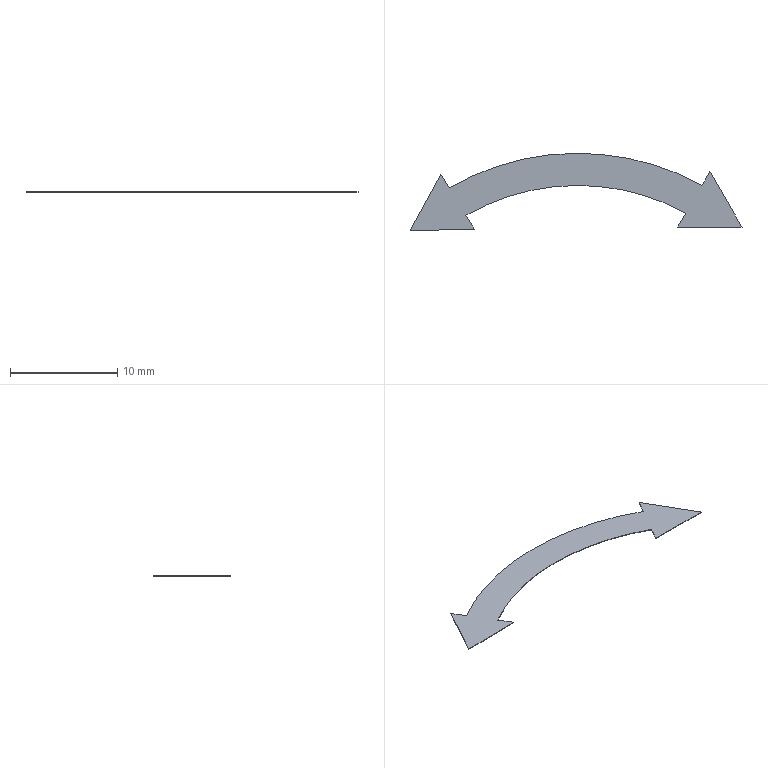Part | STEP file | J101-EBZ05-17-12-Part-1 | 1 solid | 12 faces | box 30.976 x 7.216 x 0.05 mm | volume 5.016 mm3 | plane 10 | cylinder 2 | commonest cylinder face diameters 41.852 x1 47.852 x1
STEP:
#1=CARTESIAN_POINT('',(0.,0.,0.));
#2=DIRECTION('',(0.,0.,1.));
#3=DIRECTION('',(1.,0.,0.));
#4=AXIS2_PLACEMENT_3D('',#1,#2,#3);
#5=CARTESIAN_POINT('',(12.575,12.982,0.));
#6=VERTEX_POINT('',#5);
#7=CARTESIAN_POINT('',(11.822,11.684,0.));
#8=VERTEX_POINT('',#7);
#9=CARTESIAN_POINT('',(12.575,12.982,0.));
#10=DIRECTION('',(-0.5021,-0.8648,0.));
#11=VECTOR('',#10,1.);
#12=LINE('',#9,#11);
#13=CARTESIAN_POINT('',(12.575,12.982,0.05));
#14=DIRECTION('',(0.8648,-0.5021,0.));
#15=DIRECTION('',(0.5021,0.8648,0.));
#16=AXIS2_PLACEMENT_3D('',#13,#14,#15);
#17=PLANE('',#16);
#18=CARTESIAN_POINT('',(0.,-0.05));
#19=DIRECTION('',(-1.,0.));
#20=VECTOR('',#19,1.);
#21=LINE('',#18,#20);
#22=(GEOMETRIC_REPRESENTATION_CONTEXT(2)PARAMETRIC_REPRESENTATION_CONTEXT()REPRESENTATION_CONTEXT('',''));
#23=DEFINITIONAL_REPRESENTATION('',(#21),#22);
#24=PCURVE('',#17,#23);
#25=CARTESIAN_POINT('',(0.2533,-9.259,0.));
#26=DIRECTION('',(0.,0.,1.));
#27=DIRECTION('',(1.,0.,0.));
#28=AXIS2_PLACEMENT_3D('',#25,#26,#27);
#29=PLANE('',#28);
#30=CARTESIAN_POINT('',(12.322,22.241));
#31=DIRECTION('',(-0.5021,-0.8648));
#32=VECTOR('',#31,1.);
#33=LINE('',#30,#32);
#34=(GEOMETRIC_REPRESENTATION_CONTEXT(2)PARAMETRIC_REPRESENTATION_CONTEXT()REPRESENTATION_CONTEXT('',''));
#35=DEFINITIONAL_REPRESENTATION('',(#33),#34);
#36=PCURVE('',#29,#35);
#37=SURFACE_CURVE('',#12,(#24,#36),.PCURVE_S1.);
#38=EDGE_CURVE('',#6,#8,#37,.T.);
#39=ORIENTED_EDGE('',*,*,#38,.T.);
#40=CARTESIAN_POINT('',(11.822,11.684,0.05));
#41=VERTEX_POINT('',#40);
#42=CARTESIAN_POINT('',(11.822,11.684,0.05));
#43=DIRECTION('',(0.,0.,-1.));
#44=VECTOR('',#43,1.);
#45=LINE('',#42,#44);
#46=CARTESIAN_POINT('',(-1.5,0.));
#47=DIRECTION('',(0.,-1.));
#48=VECTOR('',#47,1.);
#49=LINE('',#46,#48);
#50=(GEOMETRIC_REPRESENTATION_CONTEXT(2)PARAMETRIC_REPRESENTATION_CONTEXT()REPRESENTATION_CONTEXT('',''));
#51=DEFINITIONAL_REPRESENTATION('',(#49),#50);
#52=PCURVE('',#17,#51);
#53=CARTESIAN_POINT('',(0.2533,-9.259,0.05));
#54=DIRECTION('',(0.,0.,-1.));
#55=DIRECTION('',(-1.,0.,0.));
#56=AXIS2_PLACEMENT_3D('',#53,#54,#55);
#57=CYLINDRICAL_SURFACE('',#56,23.926);
#58=CARTESIAN_POINT('',(2.075,0.));
#59=DIRECTION('',(0.,1.));
#60=VECTOR('',#59,1.);
#61=LINE('',#58,#60);
#62=(GEOMETRIC_REPRESENTATION_CONTEXT(2)PARAMETRIC_REPRESENTATION_CONTEXT()REPRESENTATION_CONTEXT('',''));
#63=DEFINITIONAL_REPRESENTATION('',(#61),#62);
#64=PCURVE('',#57,#63);
#65=SURFACE_CURVE('',#45,(#52,#64),.PCURVE_S1.);
#66=EDGE_CURVE('',#41,#8,#65,.T.);
#67=ORIENTED_EDGE('',*,*,#66,.F.);
#68=CARTESIAN_POINT('',(12.575,12.982,0.05));
#69=VERTEX_POINT('',#68);
#70=CARTESIAN_POINT('',(12.575,12.982,0.05));
#71=DIRECTION('',(-0.5021,-0.8648,0.));
#72=VECTOR('',#71,1.);
#73=LINE('',#70,#72);
#74=CARTESIAN_POINT('',(0.,0.));
#75=DIRECTION('',(-1.,0.));
#76=VECTOR('',#75,1.);
#77=LINE('',#74,#76);
#78=(GEOMETRIC_REPRESENTATION_CONTEXT(2)PARAMETRIC_REPRESENTATION_CONTEXT()REPRESENTATION_CONTEXT('',''));
#79=DEFINITIONAL_REPRESENTATION('',(#77),#78);
#80=PCURVE('',#17,#79);
#81=CARTESIAN_POINT('',(0.2533,-9.259,0.05));
#82=DIRECTION('',(0.,0.,1.));
#83=DIRECTION('',(1.,0.,0.));
#84=AXIS2_PLACEMENT_3D('',#81,#82,#83);
#85=PLANE('',#84);
#86=CARTESIAN_POINT('',(12.322,22.241));
#87=DIRECTION('',(-0.5021,-0.8648));
#88=VECTOR('',#87,1.);
#89=LINE('',#86,#88);
#90=(GEOMETRIC_REPRESENTATION_CONTEXT(2)PARAMETRIC_REPRESENTATION_CONTEXT()REPRESENTATION_CONTEXT('',''));
#91=DEFINITIONAL_REPRESENTATION('',(#89),#90);
#92=PCURVE('',#85,#91);
#93=SURFACE_CURVE('',#73,(#80,#92),.PCURVE_S1.);
#94=EDGE_CURVE('',#69,#41,#93,.T.);
#95=ORIENTED_EDGE('',*,*,#94,.F.);
#96=CARTESIAN_POINT('',(12.575,12.982,0.05));
#97=DIRECTION('',(0.,0.,-1.));
#98=VECTOR('',#97,1.);
#99=LINE('',#96,#98);
#100=CARTESIAN_POINT('',(0.,0.));
#101=DIRECTION('',(0.,-1.));
#102=VECTOR('',#101,1.);
#103=LINE('',#100,#102);
#104=(GEOMETRIC_REPRESENTATION_CONTEXT(2)PARAMETRIC_REPRESENTATION_CONTEXT()REPRESENTATION_CONTEXT('',''));
#105=DEFINITIONAL_REPRESENTATION('',(#103),#104);
#106=PCURVE('',#17,#105);
#107=CARTESIAN_POINT('',(15.564,7.777,0.05));
#108=DIRECTION('',(-0.8672,-0.4979,0.));
#109=DIRECTION('',(0.4979,-0.8672,0.));
#110=AXIS2_PLACEMENT_3D('',#107,#108,#109);
#111=PLANE('',#110);
#112=CARTESIAN_POINT('',(-6.002,0.));
#113=DIRECTION('',(0.,-1.));
#114=VECTOR('',#113,1.);
#115=LINE('',#112,#114);
#116=(GEOMETRIC_REPRESENTATION_CONTEXT(2)PARAMETRIC_REPRESENTATION_CONTEXT()REPRESENTATION_CONTEXT('',''));
#117=DEFINITIONAL_REPRESENTATION('',(#115),#116);
#118=PCURVE('',#111,#117);
#119=SURFACE_CURVE('',#99,(#106,#118),.PCURVE_S1.);
#120=EDGE_CURVE('',#69,#6,#119,.T.);
#121=ORIENTED_EDGE('',*,*,#120,.T.);
#122=EDGE_LOOP('',(#39,#67,#95,#121));
#123=FACE_BOUND('',#122,.T.);
#124=ADVANCED_FACE('',(#123),#17,.F.);
#125=CARTESIAN_POINT('',(-11.754,11.436,0.));
#126=VERTEX_POINT('',#125);
#127=CARTESIAN_POINT('',(0.2533,-9.259,0.));
#128=DIRECTION('',(0.,0.,1.));
#129=DIRECTION('',(1.,0.,0.));
#130=AXIS2_PLACEMENT_3D('',#127,#128,#129);
#131=CIRCLE('',#130,23.926);
#132=CARTESIAN_POINT('',(3.142,0.05));
#133=DIRECTION('',(-1.,0.));
#134=VECTOR('',#133,1.);
#135=LINE('',#132,#134);
#136=(GEOMETRIC_REPRESENTATION_CONTEXT(2)PARAMETRIC_REPRESENTATION_CONTEXT()REPRESENTATION_CONTEXT('',''));
#137=DEFINITIONAL_REPRESENTATION('',(#135),#136);
#138=PCURVE('',#57,#137);
#139=CARTESIAN_POINT('',(0.,0.));
#140=DIRECTION('',(1.,0.));
#141=AXIS2_PLACEMENT_2D('',#139,#140);
#142=CIRCLE('',#141,23.926);
#143=(GEOMETRIC_REPRESENTATION_CONTEXT(2)PARAMETRIC_REPRESENTATION_CONTEXT()REPRESENTATION_CONTEXT('',''));
#144=DEFINITIONAL_REPRESENTATION('',(#142),#143);
#145=PCURVE('',#29,#144);
#146=SURFACE_CURVE('',#131,(#138,#145),.PCURVE_S1.);
#147=EDGE_CURVE('',#8,#126,#146,.T.);
#148=ORIENTED_EDGE('',*,*,#147,.T.);
#149=CARTESIAN_POINT('',(-11.754,11.436,0.05));
#150=VERTEX_POINT('',#149);
#151=CARTESIAN_POINT('',(-11.754,11.436,0.05));
#152=DIRECTION('',(0.,0.,-1.));
#153=VECTOR('',#152,1.);
#154=LINE('',#151,#153);
#155=CARTESIAN_POINT('',(1.045,0.));
#156=DIRECTION('',(0.,1.));
#157=VECTOR('',#156,1.);
#158=LINE('',#155,#157);
#159=(GEOMETRIC_REPRESENTATION_CONTEXT(2)PARAMETRIC_REPRESENTATION_CONTEXT()REPRESENTATION_CONTEXT('',''));
#160=DEFINITIONAL_REPRESENTATION('',(#158),#159);
#161=PCURVE('',#57,#160);
#162=CARTESIAN_POINT('',(-11.754,11.436,0.05));
#163=DIRECTION('',(-0.8541,-0.5202,0.));
#164=DIRECTION('',(0.5202,-0.8541,0.));
#165=AXIS2_PLACEMENT_3D('',#162,#163,#164);
#166=PLANE('',#165);
#167=CARTESIAN_POINT('',(0.,0.));
#168=DIRECTION('',(0.,-1.));
#169=VECTOR('',#168,1.);
#170=LINE('',#167,#169);
#171=(GEOMETRIC_REPRESENTATION_CONTEXT(2)PARAMETRIC_REPRESENTATION_CONTEXT()REPRESENTATION_CONTEXT('',''));
#172=DEFINITIONAL_REPRESENTATION('',(#170),#171);
#173=PCURVE('',#166,#172);
#174=SURFACE_CURVE('',#154,(#161,#173),.PCURVE_S1.);
#175=EDGE_CURVE('',#150,#126,#174,.T.);
#176=ORIENTED_EDGE('',*,*,#175,.F.);
#177=CARTESIAN_POINT('',(0.2533,-9.259,0.05));
#178=DIRECTION('',(0.,0.,1.));
#179=DIRECTION('',(1.,0.,0.));
#180=AXIS2_PLACEMENT_3D('',#177,#178,#179);
#181=CIRCLE('',#180,23.926);
#182=CARTESIAN_POINT('',(3.142,0.));
#183=DIRECTION('',(-1.,0.));
#184=VECTOR('',#183,1.);
#185=LINE('',#182,#184);
#186=(GEOMETRIC_REPRESENTATION_CONTEXT(2)PARAMETRIC_REPRESENTATION_CONTEXT()REPRESENTATION_CONTEXT('',''));
#187=DEFINITIONAL_REPRESENTATION('',(#185),#186);
#188=PCURVE('',#57,#187);
#189=CARTESIAN_POINT('',(0.,0.));
#190=DIRECTION('',(1.,0.));
#191=AXIS2_PLACEMENT_2D('',#189,#190);
#192=CIRCLE('',#191,23.926);
#193=(GEOMETRIC_REPRESENTATION_CONTEXT(2)PARAMETRIC_REPRESENTATION_CONTEXT()REPRESENTATION_CONTEXT('',''));
#194=DEFINITIONAL_REPRESENTATION('',(#192),#193);
#195=PCURVE('',#85,#194);
#196=SURFACE_CURVE('',#181,(#188,#195),.PCURVE_S1.);
#197=EDGE_CURVE('',#41,#150,#196,.T.);
#198=ORIENTED_EDGE('',*,*,#197,.F.);
#199=ORIENTED_EDGE('',*,*,#66,.T.);
#200=EDGE_LOOP('',(#148,#176,#198,#199));
#201=FACE_BOUND('',#200,.T.);
#202=ADVANCED_FACE('',(#201),#57,.T.);
#203=CARTESIAN_POINT('',(-12.535,12.717,0.));
#204=VERTEX_POINT('',#203);
#205=CARTESIAN_POINT('',(-11.754,11.436,0.));
#206=DIRECTION('',(-0.5202,0.8541,0.));
#207=VECTOR('',#206,1.);
#208=LINE('',#205,#207);
#209=CARTESIAN_POINT('',(0.,-0.05));
#210=DIRECTION('',(-1.,0.));
#211=VECTOR('',#210,1.);
#212=LINE('',#209,#211);
#213=(GEOMETRIC_REPRESENTATION_CONTEXT(2)PARAMETRIC_REPRESENTATION_CONTEXT()REPRESENTATION_CONTEXT('',''));
#214=DEFINITIONAL_REPRESENTATION('',(#212),#213);
#215=PCURVE('',#166,#214);
#216=CARTESIAN_POINT('',(-12.007,20.695));
#217=DIRECTION('',(-0.5202,0.8541));
#218=VECTOR('',#217,1.);
#219=LINE('',#216,#218);
#220=(GEOMETRIC_REPRESENTATION_CONTEXT(2)PARAMETRIC_REPRESENTATION_CONTEXT()REPRESENTATION_CONTEXT('',''));
#221=DEFINITIONAL_REPRESENTATION('',(#219),#220);
#222=PCURVE('',#29,#221);
#223=SURFACE_CURVE('',#208,(#215,#222),.PCURVE_S1.);
#224=EDGE_CURVE('',#126,#204,#223,.T.);
#225=ORIENTED_EDGE('',*,*,#224,.T.);
#226=CARTESIAN_POINT('',(-12.535,12.717,0.05));
#227=VERTEX_POINT('',#226);
#228=CARTESIAN_POINT('',(-12.535,12.717,0.05));
#229=DIRECTION('',(0.,0.,-1.));
#230=VECTOR('',#229,1.);
#231=LINE('',#228,#230);
#232=CARTESIAN_POINT('',(-1.5,0.));
#233=DIRECTION('',(0.,-1.));
#234=VECTOR('',#233,1.);
#235=LINE('',#232,#234);
#236=(GEOMETRIC_REPRESENTATION_CONTEXT(2)PARAMETRIC_REPRESENTATION_CONTEXT()REPRESENTATION_CONTEXT('',''));
#237=DEFINITIONAL_REPRESENTATION('',(#235),#236);
#238=PCURVE('',#166,#237);
#239=CARTESIAN_POINT('',(-12.535,12.717,0.05));
#240=DIRECTION('',(0.8775,-0.4795,0.));
#241=DIRECTION('',(0.4795,0.8775,0.));
#242=AXIS2_PLACEMENT_3D('',#239,#240,#241);
#243=PLANE('',#242);
#244=CARTESIAN_POINT('',(0.,0.));
#245=DIRECTION('',(0.,-1.));
#246=VECTOR('',#245,1.);
#247=LINE('',#244,#246);
#248=(GEOMETRIC_REPRESENTATION_CONTEXT(2)PARAMETRIC_REPRESENTATION_CONTEXT()REPRESENTATION_CONTEXT('',''));
#249=DEFINITIONAL_REPRESENTATION('',(#247),#248);
#250=PCURVE('',#243,#249);
#251=SURFACE_CURVE('',#231,(#238,#250),.PCURVE_S1.);
#252=EDGE_CURVE('',#227,#204,#251,.T.);
#253=ORIENTED_EDGE('',*,*,#252,.F.);
#254=CARTESIAN_POINT('',(-11.754,11.436,0.05));
#255=DIRECTION('',(-0.5202,0.8541,0.));
#256=VECTOR('',#255,1.);
#257=LINE('',#254,#256);
#258=CARTESIAN_POINT('',(0.,0.));
#259=DIRECTION('',(-1.,0.));
#260=VECTOR('',#259,1.);
#261=LINE('',#258,#260);
#262=(GEOMETRIC_REPRESENTATION_CONTEXT(2)PARAMETRIC_REPRESENTATION_CONTEXT()REPRESENTATION_CONTEXT('',''));
#263=DEFINITIONAL_REPRESENTATION('',(#261),#262);
#264=PCURVE('',#166,#263);
#265=CARTESIAN_POINT('',(-12.007,20.695));
#266=DIRECTION('',(-0.5202,0.8541));
#267=VECTOR('',#266,1.);
#268=LINE('',#265,#267);
#269=(GEOMETRIC_REPRESENTATION_CONTEXT(2)PARAMETRIC_REPRESENTATION_CONTEXT()REPRESENTATION_CONTEXT('',''));
#270=DEFINITIONAL_REPRESENTATION('',(#268),#269);
#271=PCURVE('',#85,#270);
#272=SURFACE_CURVE('',#257,(#264,#271),.PCURVE_S1.);
#273=EDGE_CURVE('',#150,#227,#272,.T.);
#274=ORIENTED_EDGE('',*,*,#273,.F.);
#275=ORIENTED_EDGE('',*,*,#175,.T.);
#276=EDGE_LOOP('',(#225,#253,#274,#275));
#277=FACE_BOUND('',#276,.T.);
#278=ADVANCED_FACE('',(#277),#166,.F.);
#279=CARTESIAN_POINT('',(-15.413,7.451,0.));
#280=VERTEX_POINT('',#279);
#281=CARTESIAN_POINT('',(-12.535,12.717,0.));
#282=DIRECTION('',(-0.4795,-0.8775,0.));
#283=VECTOR('',#282,1.);
#284=LINE('',#281,#283);
#285=CARTESIAN_POINT('',(0.,-0.05));
#286=DIRECTION('',(-1.,0.));
#287=VECTOR('',#286,1.);
#288=LINE('',#285,#287);
#289=(GEOMETRIC_REPRESENTATION_CONTEXT(2)PARAMETRIC_REPRESENTATION_CONTEXT()REPRESENTATION_CONTEXT('',''));
#290=DEFINITIONAL_REPRESENTATION('',(#288),#289);
#291=PCURVE('',#243,#290);
#292=CARTESIAN_POINT('',(-12.788,21.976));
#293=DIRECTION('',(-0.4795,-0.8775));
#294=VECTOR('',#293,1.);
#295=LINE('',#292,#294);
#296=(GEOMETRIC_REPRESENTATION_CONTEXT(2)PARAMETRIC_REPRESENTATION_CONTEXT()REPRESENTATION_CONTEXT('',''));
#297=DEFINITIONAL_REPRESENTATION('',(#295),#296);
#298=PCURVE('',#29,#297);
#299=SURFACE_CURVE('',#284,(#291,#298),.PCURVE_S1.);
#300=EDGE_CURVE('',#204,#280,#299,.T.);
#301=ORIENTED_EDGE('',*,*,#300,.T.);
#302=CARTESIAN_POINT('',(-15.413,7.451,0.05));
#303=VERTEX_POINT('',#302);
#304=CARTESIAN_POINT('',(-15.413,7.451,0.05));
#305=DIRECTION('',(0.,0.,-1.));
#306=VECTOR('',#305,1.);
#307=LINE('',#304,#306);
#308=CARTESIAN_POINT('',(-6.002,0.));
#309=DIRECTION('',(0.,-1.));
#310=VECTOR('',#309,1.);
#311=LINE('',#308,#310);
#312=(GEOMETRIC_REPRESENTATION_CONTEXT(2)PARAMETRIC_REPRESENTATION_CONTEXT()REPRESENTATION_CONTEXT('',''));
#313=DEFINITIONAL_REPRESENTATION('',(#311),#312);
#314=PCURVE('',#243,#313);
#315=CARTESIAN_POINT('',(-15.413,7.451,0.05));
#316=DIRECTION('',(-0.02346,0.9997,0.));
#317=DIRECTION('',(-0.9997,-0.02346,0.));
#318=AXIS2_PLACEMENT_3D('',#315,#316,#317);
#319=PLANE('',#318);
#320=CARTESIAN_POINT('',(0.,0.));
#321=DIRECTION('',(0.,-1.));
#322=VECTOR('',#321,1.);
#323=LINE('',#320,#322);
#324=(GEOMETRIC_REPRESENTATION_CONTEXT(2)PARAMETRIC_REPRESENTATION_CONTEXT()REPRESENTATION_CONTEXT('',''));
#325=DEFINITIONAL_REPRESENTATION('',(#323),#324);
#326=PCURVE('',#319,#325);
#327=SURFACE_CURVE('',#307,(#314,#326),.PCURVE_S1.);
#328=EDGE_CURVE('',#303,#280,#327,.T.);
#329=ORIENTED_EDGE('',*,*,#328,.F.);
#330=CARTESIAN_POINT('',(-12.535,12.717,0.05));
#331=DIRECTION('',(-0.4795,-0.8775,0.));
#332=VECTOR('',#331,1.);
#333=LINE('',#330,#332);
#334=CARTESIAN_POINT('',(0.,0.));
#335=DIRECTION('',(-1.,0.));
#336=VECTOR('',#335,1.);
#337=LINE('',#334,#336);
#338=(GEOMETRIC_REPRESENTATION_CONTEXT(2)PARAMETRIC_REPRESENTATION_CONTEXT()REPRESENTATION_CONTEXT('',''));
#339=DEFINITIONAL_REPRESENTATION('',(#337),#338);
#340=PCURVE('',#243,#339);
#341=CARTESIAN_POINT('',(-12.788,21.976));
#342=DIRECTION('',(-0.4795,-0.8775));
#343=VECTOR('',#342,1.);
#344=LINE('',#341,#343);
#345=(GEOMETRIC_REPRESENTATION_CONTEXT(2)PARAMETRIC_REPRESENTATION_CONTEXT()REPRESENTATION_CONTEXT('',''));
#346=DEFINITIONAL_REPRESENTATION('',(#344),#345);
#347=PCURVE('',#85,#346);
#348=SURFACE_CURVE('',#333,(#340,#347),.PCURVE_S1.);
#349=EDGE_CURVE('',#227,#303,#348,.T.);
#350=ORIENTED_EDGE('',*,*,#349,.F.);
#351=ORIENTED_EDGE('',*,*,#252,.T.);
#352=EDGE_LOOP('',(#301,#329,#350,#351));
#353=FACE_BOUND('',#352,.T.);
#354=ADVANCED_FACE('',(#353),#243,.F.);
#355=CARTESIAN_POINT('',(-9.413,7.592,0.));
#356=VERTEX_POINT('',#355);
#357=CARTESIAN_POINT('',(-15.413,7.451,0.));
#358=DIRECTION('',(0.9997,0.02346,0.));
#359=VECTOR('',#358,1.);
#360=LINE('',#357,#359);
#361=CARTESIAN_POINT('',(0.,-0.05));
#362=DIRECTION('',(-1.,0.));
#363=VECTOR('',#362,1.);
#364=LINE('',#361,#363);
#365=(GEOMETRIC_REPRESENTATION_CONTEXT(2)PARAMETRIC_REPRESENTATION_CONTEXT()REPRESENTATION_CONTEXT('',''));
#366=DEFINITIONAL_REPRESENTATION('',(#364),#365);
#367=PCURVE('',#319,#366);
#368=CARTESIAN_POINT('',(-15.666,16.71));
#369=DIRECTION('',(0.9997,0.02346));
#370=VECTOR('',#369,1.);
#371=LINE('',#368,#370);
#372=(GEOMETRIC_REPRESENTATION_CONTEXT(2)PARAMETRIC_REPRESENTATION_CONTEXT()REPRESENTATION_CONTEXT('',''));
#373=DEFINITIONAL_REPRESENTATION('',(#371),#372);
#374=PCURVE('',#29,#373);
#375=SURFACE_CURVE('',#360,(#367,#374),.PCURVE_S1.);
#376=EDGE_CURVE('',#280,#356,#375,.T.);
#377=ORIENTED_EDGE('',*,*,#376,.T.);
#378=CARTESIAN_POINT('',(-9.413,7.592,0.05));
#379=VERTEX_POINT('',#378);
#380=CARTESIAN_POINT('',(-9.413,7.592,0.05));
#381=DIRECTION('',(0.,0.,-1.));
#382=VECTOR('',#381,1.);
#383=LINE('',#380,#382);
#384=CARTESIAN_POINT('',(-6.002,0.));
#385=DIRECTION('',(0.,-1.));
#386=VECTOR('',#385,1.);
#387=LINE('',#384,#386);
#388=(GEOMETRIC_REPRESENTATION_CONTEXT(2)PARAMETRIC_REPRESENTATION_CONTEXT()REPRESENTATION_CONTEXT('',''));
#389=DEFINITIONAL_REPRESENTATION('',(#387),#388);
#390=PCURVE('',#319,#389);
#391=CARTESIAN_POINT('',(-9.413,7.592,0.05));
#392=DIRECTION('',(-0.8541,-0.5202,0.));
#393=DIRECTION('',(0.5202,-0.8541,0.));
#394=AXIS2_PLACEMENT_3D('',#391,#392,#393);
#395=PLANE('',#394);
#396=CARTESIAN_POINT('',(0.,0.));
#397=DIRECTION('',(0.,-1.));
#398=VECTOR('',#397,1.);
#399=LINE('',#396,#398);
#400=(GEOMETRIC_REPRESENTATION_CONTEXT(2)PARAMETRIC_REPRESENTATION_CONTEXT()REPRESENTATION_CONTEXT('',''));
#401=DEFINITIONAL_REPRESENTATION('',(#399),#400);
#402=PCURVE('',#395,#401);
#403=SURFACE_CURVE('',#383,(#390,#402),.PCURVE_S1.);
#404=EDGE_CURVE('',#379,#356,#403,.T.);
#405=ORIENTED_EDGE('',*,*,#404,.F.);
#406=CARTESIAN_POINT('',(-15.413,7.451,0.05));
#407=DIRECTION('',(0.9997,0.02346,0.));
#408=VECTOR('',#407,1.);
#409=LINE('',#406,#408);
#410=CARTESIAN_POINT('',(0.,0.));
#411=DIRECTION('',(-1.,0.));
#412=VECTOR('',#411,1.);
#413=LINE('',#410,#412);
#414=(GEOMETRIC_REPRESENTATION_CONTEXT(2)PARAMETRIC_REPRESENTATION_CONTEXT()REPRESENTATION_CONTEXT('',''));
#415=DEFINITIONAL_REPRESENTATION('',(#413),#414);
#416=PCURVE('',#319,#415);
#417=CARTESIAN_POINT('',(-15.666,16.71));
#418=DIRECTION('',(0.9997,0.02346));
#419=VECTOR('',#418,1.);
#420=LINE('',#417,#419);
#421=(GEOMETRIC_REPRESENTATION_CONTEXT(2)PARAMETRIC_REPRESENTATION_CONTEXT()REPRESENTATION_CONTEXT('',''));
#422=DEFINITIONAL_REPRESENTATION('',(#420),#421);
#423=PCURVE('',#85,#422);
#424=SURFACE_CURVE('',#409,(#416,#423),.PCURVE_S1.);
#425=EDGE_CURVE('',#303,#379,#424,.T.);
#426=ORIENTED_EDGE('',*,*,#425,.F.);
#427=ORIENTED_EDGE('',*,*,#328,.T.);
#428=EDGE_LOOP('',(#377,#405,#426,#427));
#429=FACE_BOUND('',#428,.T.);
#430=ADVANCED_FACE('',(#429),#319,.F.);
#431=CARTESIAN_POINT('',(-10.193,8.873,0.));
#432=VERTEX_POINT('',#431);
#433=CARTESIAN_POINT('',(-9.413,7.592,0.));
#434=DIRECTION('',(-0.5202,0.8541,0.));
#435=VECTOR('',#434,1.);
#436=LINE('',#433,#435);
#437=CARTESIAN_POINT('',(0.,-0.05));
#438=DIRECTION('',(-1.,0.));
#439=VECTOR('',#438,1.);
#440=LINE('',#437,#439);
#441=(GEOMETRIC_REPRESENTATION_CONTEXT(2)PARAMETRIC_REPRESENTATION_CONTEXT()REPRESENTATION_CONTEXT('',''));
#442=DEFINITIONAL_REPRESENTATION('',(#440),#441);
#443=PCURVE('',#395,#442);
#444=CARTESIAN_POINT('',(-9.666,16.851));
#445=DIRECTION('',(-0.5202,0.8541));
#446=VECTOR('',#445,1.);
#447=LINE('',#444,#446);
#448=(GEOMETRIC_REPRESENTATION_CONTEXT(2)PARAMETRIC_REPRESENTATION_CONTEXT()REPRESENTATION_CONTEXT('',''));
#449=DEFINITIONAL_REPRESENTATION('',(#447),#448);
#450=PCURVE('',#29,#449);
#451=SURFACE_CURVE('',#436,(#443,#450),.PCURVE_S1.);
#452=EDGE_CURVE('',#356,#432,#451,.T.);
#453=ORIENTED_EDGE('',*,*,#452,.T.);
#454=CARTESIAN_POINT('',(-10.193,8.873,0.05));
#455=VERTEX_POINT('',#454);
#456=CARTESIAN_POINT('',(-10.193,8.873,0.05));
#457=DIRECTION('',(0.,0.,-1.));
#458=VECTOR('',#457,1.);
#459=LINE('',#456,#458);
#460=CARTESIAN_POINT('',(-1.5,0.));
#461=DIRECTION('',(0.,-1.));
#462=VECTOR('',#461,1.);
#463=LINE('',#460,#462);
#464=(GEOMETRIC_REPRESENTATION_CONTEXT(2)PARAMETRIC_REPRESENTATION_CONTEXT()REPRESENTATION_CONTEXT('',''));
#465=DEFINITIONAL_REPRESENTATION('',(#463),#464);
#466=PCURVE('',#395,#465);
#467=CARTESIAN_POINT('',(0.2533,-9.259,0.05));
#468=DIRECTION('',(0.,0.,-1.));
#469=DIRECTION('',(-1.,0.,0.));
#470=AXIS2_PLACEMENT_3D('',#467,#468,#469);
#471=CYLINDRICAL_SURFACE('',#470,20.926);
#472=CARTESIAN_POINT('',(1.048,0.));
#473=DIRECTION('',(0.,1.));
#474=VECTOR('',#473,1.);
#475=LINE('',#472,#474);
#476=(GEOMETRIC_REPRESENTATION_CONTEXT(2)PARAMETRIC_REPRESENTATION_CONTEXT()REPRESENTATION_CONTEXT('',''));
#477=DEFINITIONAL_REPRESENTATION('',(#475),#476);
#478=PCURVE('',#471,#477);
#479=SURFACE_CURVE('',#459,(#466,#478),.PCURVE_S1.);
#480=EDGE_CURVE('',#455,#432,#479,.T.);
#481=ORIENTED_EDGE('',*,*,#480,.F.);
#482=CARTESIAN_POINT('',(-9.413,7.592,0.05));
#483=DIRECTION('',(-0.5202,0.8541,0.));
#484=VECTOR('',#483,1.);
#485=LINE('',#482,#484);
#486=CARTESIAN_POINT('',(0.,0.));
#487=DIRECTION('',(-1.,0.));
#488=VECTOR('',#487,1.);
#489=LINE('',#486,#488);
#490=(GEOMETRIC_REPRESENTATION_CONTEXT(2)PARAMETRIC_REPRESENTATION_CONTEXT()REPRESENTATION_CONTEXT('',''));
#491=DEFINITIONAL_REPRESENTATION('',(#489),#490);
#492=PCURVE('',#395,#491);
#493=CARTESIAN_POINT('',(-9.666,16.851));
#494=DIRECTION('',(-0.5202,0.8541));
#495=VECTOR('',#494,1.);
#496=LINE('',#493,#495);
#497=(GEOMETRIC_REPRESENTATION_CONTEXT(2)PARAMETRIC_REPRESENTATION_CONTEXT()REPRESENTATION_CONTEXT('',''));
#498=DEFINITIONAL_REPRESENTATION('',(#496),#497);
#499=PCURVE('',#85,#498);
#500=SURFACE_CURVE('',#485,(#492,#499),.PCURVE_S1.);
#501=EDGE_CURVE('',#379,#455,#500,.T.);
#502=ORIENTED_EDGE('',*,*,#501,.F.);
#503=ORIENTED_EDGE('',*,*,#404,.T.);
#504=EDGE_LOOP('',(#453,#481,#502,#503));
#505=FACE_BOUND('',#504,.T.);
#506=ADVANCED_FACE('',(#505),#395,.F.);
#507=ORIENTED_EDGE('',*,*,#480,.F.);
#508=CARTESIAN_POINT('',(10.315,9.089,0.05));
#509=VERTEX_POINT('',#508);
#510=CARTESIAN_POINT('',(0.2533,-9.259,0.05));
#511=DIRECTION('',(0.,0.,-1.));
#512=DIRECTION('',(-1.,0.,0.));
#513=AXIS2_PLACEMENT_3D('',#510,#511,#512);
#514=CIRCLE('',#513,20.926);
#515=CARTESIAN_POINT('',(0.,0.));
#516=DIRECTION('',(1.,0.));
#517=VECTOR('',#516,1.);
#518=LINE('',#515,#517);
#519=(GEOMETRIC_REPRESENTATION_CONTEXT(2)PARAMETRIC_REPRESENTATION_CONTEXT()REPRESENTATION_CONTEXT('',''));
#520=DEFINITIONAL_REPRESENTATION('',(#518),#519);
#521=PCURVE('',#471,#520);
#522=CARTESIAN_POINT('',(-20.926,0.));
#523=CARTESIAN_POINT('',(-20.926,36.245));
#524=CARTESIAN_POINT('',(10.463,18.123));
#525=CARTESIAN_POINT('',(41.852,0.));
#526=CARTESIAN_POINT('',(10.463,-18.123));
#527=CARTESIAN_POINT('',(-20.926,-36.245));
#528=CARTESIAN_POINT('',(-20.926,0.));
#529=(BOUNDED_CURVE()B_SPLINE_CURVE(2,(#522,#523,#524,#525,#526,#527,#528),.UNSPECIFIED.,.T.,.F.)B_SPLINE_CURVE_WITH_KNOTS((1,2,2,2,2,1),(-2.094,0.,2.094,4.189,6.283,8.378),.UNSPECIFIED.)CURVE()GEOMETRIC_REPRESENTATION_ITEM()RATIONAL_B_SPLINE_CURVE((1.,0.5,1.,0.5,1.,0.5,1.))REPRESENTATION_ITEM(''));
#530=(GEOMETRIC_REPRESENTATION_CONTEXT(2)PARAMETRIC_REPRESENTATION_CONTEXT()REPRESENTATION_CONTEXT('',''));
#531=DEFINITIONAL_REPRESENTATION('',(#529),#530);
#532=PCURVE('',#85,#531);
#533=SURFACE_CURVE('',#514,(#521,#532),.PCURVE_S1.);
#534=EDGE_CURVE('',#455,#509,#533,.T.);
#535=ORIENTED_EDGE('',*,*,#534,.T.);
#536=CARTESIAN_POINT('',(10.315,9.089,0.));
#537=VERTEX_POINT('',#536);
#538=CARTESIAN_POINT('',(10.315,9.089,0.05));
#539=DIRECTION('',(0.,0.,-1.));
#540=VECTOR('',#539,1.);
#541=LINE('',#538,#540);
#542=CARTESIAN_POINT('',(2.072,0.));
#543=DIRECTION('',(0.,1.));
#544=VECTOR('',#543,1.);
#545=LINE('',#542,#544);
#546=(GEOMETRIC_REPRESENTATION_CONTEXT(2)PARAMETRIC_REPRESENTATION_CONTEXT()REPRESENTATION_CONTEXT('',''));
#547=DEFINITIONAL_REPRESENTATION('',(#545),#546);
#548=PCURVE('',#471,#547);
#549=CARTESIAN_POINT('',(10.315,9.089,0.05));
#550=DIRECTION('',(0.8648,-0.5021,0.));
#551=DIRECTION('',(0.5021,0.8648,0.));
#552=AXIS2_PLACEMENT_3D('',#549,#550,#551);
#553=PLANE('',#552);
#554=CARTESIAN_POINT('',(0.,0.));
#555=DIRECTION('',(0.,-1.));
#556=VECTOR('',#555,1.);
#557=LINE('',#554,#556);
#558=(GEOMETRIC_REPRESENTATION_CONTEXT(2)PARAMETRIC_REPRESENTATION_CONTEXT()REPRESENTATION_CONTEXT('',''));
#559=DEFINITIONAL_REPRESENTATION('',(#557),#558);
#560=PCURVE('',#553,#559);
#561=SURFACE_CURVE('',#541,(#548,#560),.PCURVE_S1.);
#562=EDGE_CURVE('',#509,#537,#561,.T.);
#563=ORIENTED_EDGE('',*,*,#562,.T.);
#564=CARTESIAN_POINT('',(0.2533,-9.259,0.));
#565=DIRECTION('',(0.,0.,-1.));
#566=DIRECTION('',(-1.,0.,0.));
#567=AXIS2_PLACEMENT_3D('',#564,#565,#566);
#568=CIRCLE('',#567,20.926);
#569=CARTESIAN_POINT('',(0.,0.05));
#570=DIRECTION('',(1.,0.));
#571=VECTOR('',#570,1.);
#572=LINE('',#569,#571);
#573=(GEOMETRIC_REPRESENTATION_CONTEXT(2)PARAMETRIC_REPRESENTATION_CONTEXT()REPRESENTATION_CONTEXT('',''));
#574=DEFINITIONAL_REPRESENTATION('',(#572),#573);
#575=PCURVE('',#471,#574);
#576=CARTESIAN_POINT('',(-20.926,0.));
#577=CARTESIAN_POINT('',(-20.926,36.245));
#578=CARTESIAN_POINT('',(10.463,18.123));
#579=CARTESIAN_POINT('',(41.852,0.));
#580=CARTESIAN_POINT('',(10.463,-18.123));
#581=CARTESIAN_POINT('',(-20.926,-36.245));
#582=CARTESIAN_POINT('',(-20.926,0.));
#583=(BOUNDED_CURVE()B_SPLINE_CURVE(2,(#576,#577,#578,#579,#580,#581,#582),.UNSPECIFIED.,.T.,.F.)B_SPLINE_CURVE_WITH_KNOTS((1,2,2,2,2,1),(-2.094,0.,2.094,4.189,6.283,8.378),.UNSPECIFIED.)CURVE()GEOMETRIC_REPRESENTATION_ITEM()RATIONAL_B_SPLINE_CURVE((1.,0.5,1.,0.5,1.,0.5,1.))REPRESENTATION_ITEM(''));
#584=(GEOMETRIC_REPRESENTATION_CONTEXT(2)PARAMETRIC_REPRESENTATION_CONTEXT()REPRESENTATION_CONTEXT('',''));
#585=DEFINITIONAL_REPRESENTATION('',(#583),#584);
#586=PCURVE('',#29,#585);
#587=SURFACE_CURVE('',#568,(#575,#586),.PCURVE_S1.);
#588=EDGE_CURVE('',#432,#537,#587,.T.);
#589=ORIENTED_EDGE('',*,*,#588,.F.);
#590=EDGE_LOOP('',(#507,#535,#563,#589));
#591=FACE_BOUND('',#590,.F.);
#592=ADVANCED_FACE('',(#591),#471,.F.);
#593=CARTESIAN_POINT('',(9.562,7.792,0.));
#594=VERTEX_POINT('',#593);
#595=CARTESIAN_POINT('',(10.315,9.089,0.));
#596=DIRECTION('',(-0.5021,-0.8648,0.));
#597=VECTOR('',#596,1.);
#598=LINE('',#595,#597);
#599=CARTESIAN_POINT('',(0.,-0.05));
#600=DIRECTION('',(-1.,0.));
#601=VECTOR('',#600,1.);
#602=LINE('',#599,#601);
#603=(GEOMETRIC_REPRESENTATION_CONTEXT(2)PARAMETRIC_REPRESENTATION_CONTEXT()REPRESENTATION_CONTEXT('',''));
#604=DEFINITIONAL_REPRESENTATION('',(#602),#603);
#605=PCURVE('',#553,#604);
#606=CARTESIAN_POINT('',(10.062,18.348));
#607=DIRECTION('',(-0.5021,-0.8648));
#608=VECTOR('',#607,1.);
#609=LINE('',#606,#608);
#610=(GEOMETRIC_REPRESENTATION_CONTEXT(2)PARAMETRIC_REPRESENTATION_CONTEXT()REPRESENTATION_CONTEXT('',''));
#611=DEFINITIONAL_REPRESENTATION('',(#609),#610);
#612=PCURVE('',#29,#611);
#613=SURFACE_CURVE('',#598,(#605,#612),.PCURVE_S1.);
#614=EDGE_CURVE('',#537,#594,#613,.T.);
#615=ORIENTED_EDGE('',*,*,#614,.T.);
#616=CARTESIAN_POINT('',(9.562,7.792,0.05));
#617=VERTEX_POINT('',#616);
#618=CARTESIAN_POINT('',(9.562,7.792,0.05));
#619=DIRECTION('',(0.,0.,-1.));
#620=VECTOR('',#619,1.);
#621=LINE('',#618,#620);
#622=CARTESIAN_POINT('',(-1.5,0.));
#623=DIRECTION('',(0.,-1.));
#624=VECTOR('',#623,1.);
#625=LINE('',#622,#624);
#626=(GEOMETRIC_REPRESENTATION_CONTEXT(2)PARAMETRIC_REPRESENTATION_CONTEXT()REPRESENTATION_CONTEXT('',''));
#627=DEFINITIONAL_REPRESENTATION('',(#625),#626);
#628=PCURVE('',#553,#627);
#629=CARTESIAN_POINT('',(9.562,7.792,0.05));
#630=DIRECTION('',(0.002387,1.,0.));
#631=DIRECTION('',(-1.,0.002387,0.));
#632=AXIS2_PLACEMENT_3D('',#629,#630,#631);
#633=PLANE('',#632);
#634=CARTESIAN_POINT('',(0.,0.));
#635=DIRECTION('',(0.,-1.));
#636=VECTOR('',#635,1.);
#637=LINE('',#634,#636);
#638=(GEOMETRIC_REPRESENTATION_CONTEXT(2)PARAMETRIC_REPRESENTATION_CONTEXT()REPRESENTATION_CONTEXT('',''));
#639=DEFINITIONAL_REPRESENTATION('',(#637),#638);
#640=PCURVE('',#633,#639);
#641=SURFACE_CURVE('',#621,(#628,#640),.PCURVE_S1.);
#642=EDGE_CURVE('',#617,#594,#641,.T.);
#643=ORIENTED_EDGE('',*,*,#642,.F.);
#644=CARTESIAN_POINT('',(10.315,9.089,0.05));
#645=DIRECTION('',(-0.5021,-0.8648,0.));
#646=VECTOR('',#645,1.);
#647=LINE('',#644,#646);
#648=CARTESIAN_POINT('',(0.,0.));
#649=DIRECTION('',(-1.,0.));
#650=VECTOR('',#649,1.);
#651=LINE('',#648,#650);
#652=(GEOMETRIC_REPRESENTATION_CONTEXT(2)PARAMETRIC_REPRESENTATION_CONTEXT()REPRESENTATION_CONTEXT('',''));
#653=DEFINITIONAL_REPRESENTATION('',(#651),#652);
#654=PCURVE('',#553,#653);
#655=CARTESIAN_POINT('',(10.062,18.348));
#656=DIRECTION('',(-0.5021,-0.8648));
#657=VECTOR('',#656,1.);
#658=LINE('',#655,#657);
#659=(GEOMETRIC_REPRESENTATION_CONTEXT(2)PARAMETRIC_REPRESENTATION_CONTEXT()REPRESENTATION_CONTEXT('',''));
#660=DEFINITIONAL_REPRESENTATION('',(#658),#659);
#661=PCURVE('',#85,#660);
#662=SURFACE_CURVE('',#647,(#654,#661),.PCURVE_S1.);
#663=EDGE_CURVE('',#509,#617,#662,.T.);
#664=ORIENTED_EDGE('',*,*,#663,.F.);
#665=ORIENTED_EDGE('',*,*,#562,.T.);
#666=EDGE_LOOP('',(#615,#643,#664,#665));
#667=FACE_BOUND('',#666,.T.);
#668=ADVANCED_FACE('',(#667),#553,.F.);
#669=CARTESIAN_POINT('',(15.564,7.777,0.));
#670=VERTEX_POINT('',#669);
#671=CARTESIAN_POINT('',(9.562,7.792,0.));
#672=DIRECTION('',(1.,-0.002387,0.));
#673=VECTOR('',#672,1.);
#674=LINE('',#671,#673);
#675=CARTESIAN_POINT('',(0.,-0.05));
#676=DIRECTION('',(-1.,0.));
#677=VECTOR('',#676,1.);
#678=LINE('',#675,#677);
#679=(GEOMETRIC_REPRESENTATION_CONTEXT(2)PARAMETRIC_REPRESENTATION_CONTEXT()REPRESENTATION_CONTEXT('',''));
#680=DEFINITIONAL_REPRESENTATION('',(#678),#679);
#681=PCURVE('',#633,#680);
#682=CARTESIAN_POINT('',(9.309,17.051));
#683=DIRECTION('',(1.,-0.002387));
#684=VECTOR('',#683,1.);
#685=LINE('',#682,#684);
#686=(GEOMETRIC_REPRESENTATION_CONTEXT(2)PARAMETRIC_REPRESENTATION_CONTEXT()REPRESENTATION_CONTEXT('',''));
#687=DEFINITIONAL_REPRESENTATION('',(#685),#686);
#688=PCURVE('',#29,#687);
#689=SURFACE_CURVE('',#674,(#681,#688),.PCURVE_S1.);
#690=EDGE_CURVE('',#594,#670,#689,.T.);
#691=ORIENTED_EDGE('',*,*,#690,.T.);
#692=CARTESIAN_POINT('',(15.564,7.777,0.05));
#693=VERTEX_POINT('',#692);
#694=CARTESIAN_POINT('',(15.564,7.777,0.05));
#695=DIRECTION('',(0.,0.,-1.));
#696=VECTOR('',#695,1.);
#697=LINE('',#694,#696);
#698=CARTESIAN_POINT('',(-6.002,0.));
#699=DIRECTION('',(0.,-1.));
#700=VECTOR('',#699,1.);
#701=LINE('',#698,#700);
#702=(GEOMETRIC_REPRESENTATION_CONTEXT(2)PARAMETRIC_REPRESENTATION_CONTEXT()REPRESENTATION_CONTEXT('',''));
#703=DEFINITIONAL_REPRESENTATION('',(#701),#702);
#704=PCURVE('',#633,#703);
#705=CARTESIAN_POINT('',(0.,0.));
#706=DIRECTION('',(0.,-1.));
#707=VECTOR('',#706,1.);
#708=LINE('',#705,#707);
#709=(GEOMETRIC_REPRESENTATION_CONTEXT(2)PARAMETRIC_REPRESENTATION_CONTEXT()REPRESENTATION_CONTEXT('',''));
#710=DEFINITIONAL_REPRESENTATION('',(#708),#709);
#711=PCURVE('',#111,#710);
#712=SURFACE_CURVE('',#697,(#704,#711),.PCURVE_S1.);
#713=EDGE_CURVE('',#693,#670,#712,.T.);
#714=ORIENTED_EDGE('',*,*,#713,.F.);
#715=CARTESIAN_POINT('',(9.562,7.792,0.05));
#716=DIRECTION('',(1.,-0.002387,0.));
#717=VECTOR('',#716,1.);
#718=LINE('',#715,#717);
#719=CARTESIAN_POINT('',(0.,0.));
#720=DIRECTION('',(-1.,0.));
#721=VECTOR('',#720,1.);
#722=LINE('',#719,#721);
#723=(GEOMETRIC_REPRESENTATION_CONTEXT(2)PARAMETRIC_REPRESENTATION_CONTEXT()REPRESENTATION_CONTEXT('',''));
#724=DEFINITIONAL_REPRESENTATION('',(#722),#723);
#725=PCURVE('',#633,#724);
#726=CARTESIAN_POINT('',(9.309,17.051));
#727=DIRECTION('',(1.,-0.002387));
#728=VECTOR('',#727,1.);
#729=LINE('',#726,#728);
#730=(GEOMETRIC_REPRESENTATION_CONTEXT(2)PARAMETRIC_REPRESENTATION_CONTEXT()REPRESENTATION_CONTEXT('',''));
#731=DEFINITIONAL_REPRESENTATION('',(#729),#730);
#732=PCURVE('',#85,#731);
#733=SURFACE_CURVE('',#718,(#725,#732),.PCURVE_S1.);
#734=EDGE_CURVE('',#617,#693,#733,.T.);
#735=ORIENTED_EDGE('',*,*,#734,.F.);
#736=ORIENTED_EDGE('',*,*,#642,.T.);
#737=EDGE_LOOP('',(#691,#714,#735,#736));
#738=FACE_BOUND('',#737,.T.);
#739=ADVANCED_FACE('',(#738),#633,.F.);
#740=CARTESIAN_POINT('',(15.564,7.777,0.));
#741=DIRECTION('',(-0.4979,0.8672,0.));
#742=VECTOR('',#741,1.);
#743=LINE('',#740,#742);
#744=CARTESIAN_POINT('',(0.,-0.05));
#745=DIRECTION('',(-1.,0.));
#746=VECTOR('',#745,1.);
#747=LINE('',#744,#746);
#748=(GEOMETRIC_REPRESENTATION_CONTEXT(2)PARAMETRIC_REPRESENTATION_CONTEXT()REPRESENTATION_CONTEXT('',''));
#749=DEFINITIONAL_REPRESENTATION('',(#747),#748);
#750=PCURVE('',#111,#749);
#751=CARTESIAN_POINT('',(15.31,17.036));
#752=DIRECTION('',(-0.4979,0.8672));
#753=VECTOR('',#752,1.);
#754=LINE('',#751,#753);
#755=(GEOMETRIC_REPRESENTATION_CONTEXT(2)PARAMETRIC_REPRESENTATION_CONTEXT()REPRESENTATION_CONTEXT('',''));
#756=DEFINITIONAL_REPRESENTATION('',(#754),#755);
#757=PCURVE('',#29,#756);
#758=SURFACE_CURVE('',#743,(#750,#757),.PCURVE_S1.);
#759=EDGE_CURVE('',#670,#6,#758,.T.);
#760=ORIENTED_EDGE('',*,*,#759,.T.);
#761=ORIENTED_EDGE('',*,*,#120,.F.);
#762=CARTESIAN_POINT('',(15.564,7.777,0.05));
#763=DIRECTION('',(-0.4979,0.8672,0.));
#764=VECTOR('',#763,1.);
#765=LINE('',#762,#764);
#766=CARTESIAN_POINT('',(0.,0.));
#767=DIRECTION('',(-1.,0.));
#768=VECTOR('',#767,1.);
#769=LINE('',#766,#768);
#770=(GEOMETRIC_REPRESENTATION_CONTEXT(2)PARAMETRIC_REPRESENTATION_CONTEXT()REPRESENTATION_CONTEXT('',''));
#771=DEFINITIONAL_REPRESENTATION('',(#769),#770);
#772=PCURVE('',#111,#771);
#773=CARTESIAN_POINT('',(15.31,17.036));
#774=DIRECTION('',(-0.4979,0.8672));
#775=VECTOR('',#774,1.);
#776=LINE('',#773,#775);
#777=(GEOMETRIC_REPRESENTATION_CONTEXT(2)PARAMETRIC_REPRESENTATION_CONTEXT()REPRESENTATION_CONTEXT('',''));
#778=DEFINITIONAL_REPRESENTATION('',(#776),#777);
#779=PCURVE('',#85,#778);
#780=SURFACE_CURVE('',#765,(#772,#779),.PCURVE_S1.);
#781=EDGE_CURVE('',#693,#69,#780,.T.);
#782=ORIENTED_EDGE('',*,*,#781,.F.);
#783=ORIENTED_EDGE('',*,*,#713,.T.);
#784=EDGE_LOOP('',(#760,#761,#782,#783));
#785=FACE_BOUND('',#784,.T.);
#786=ADVANCED_FACE('',(#785),#111,.F.);
#787=ORIENTED_EDGE('',*,*,#94,.T.);
#788=ORIENTED_EDGE('',*,*,#197,.T.);
#789=ORIENTED_EDGE('',*,*,#273,.T.);
#790=ORIENTED_EDGE('',*,*,#349,.T.);
#791=ORIENTED_EDGE('',*,*,#425,.T.);
#792=ORIENTED_EDGE('',*,*,#501,.T.);
#793=ORIENTED_EDGE('',*,*,#534,.T.);
#794=ORIENTED_EDGE('',*,*,#663,.T.);
#795=ORIENTED_EDGE('',*,*,#734,.T.);
#796=ORIENTED_EDGE('',*,*,#781,.T.);
#797=EDGE_LOOP('',(#787,#788,#789,#790,#791,#792,#793,#794,#795,#796));
#798=FACE_BOUND('',#797,.T.);
#799=ADVANCED_FACE('',(#798),#85,.T.);
#800=ORIENTED_EDGE('',*,*,#38,.F.);
#801=ORIENTED_EDGE('',*,*,#759,.F.);
#802=ORIENTED_EDGE('',*,*,#690,.F.);
#803=ORIENTED_EDGE('',*,*,#614,.F.);
#804=ORIENTED_EDGE('',*,*,#588,.F.);
#805=ORIENTED_EDGE('',*,*,#452,.F.);
#806=ORIENTED_EDGE('',*,*,#376,.F.);
#807=ORIENTED_EDGE('',*,*,#300,.F.);
#808=ORIENTED_EDGE('',*,*,#224,.F.);
#809=ORIENTED_EDGE('',*,*,#147,.F.);
#810=EDGE_LOOP('',(#800,#801,#802,#803,#804,#805,#806,#807,#808,#809));
#811=FACE_BOUND('',#810,.T.);
#812=ADVANCED_FACE('',(#811),#29,.F.);
#813=CLOSED_SHELL('',(#124,#202,#278,#354,#430,#506,#592,#668,#739,#786,#799,#812));
#814=MANIFOLD_SOLID_BREP('',#813);
#815=(LENGTH_UNIT()NAMED_UNIT(*)SI_UNIT(.MILLI.,.METRE.));
#816=UNCERTAINTY_MEASURE_WITH_UNIT(LENGTH_MEASURE(0.0000001),#815,'','');
#817=(NAMED_UNIT(*)PLANE_ANGLE_UNIT()SI_UNIT($,.RADIAN.));
#818=(NAMED_UNIT(*)SI_UNIT($,.STERADIAN.)SOLID_ANGLE_UNIT());
#819=(GEOMETRIC_REPRESENTATION_CONTEXT(3)GLOBAL_UNCERTAINTY_ASSIGNED_CONTEXT((#816))GLOBAL_UNIT_ASSIGNED_CONTEXT((#815,#817,#818))REPRESENTATION_CONTEXT('',''));
#820=ADVANCED_BREP_SHAPE_REPRESENTATION('',(#4,#814),#819);